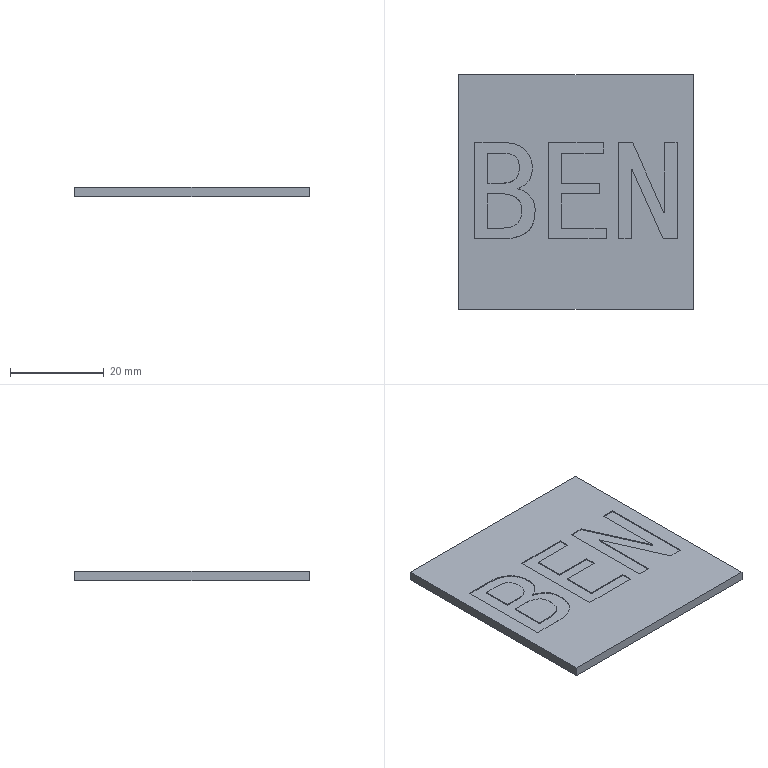Part | STEP file | lll_id1306_x_t | 1 solid | 45 faces | box 50 x 50 x 2 mm | volume 4916 mm3 | plane 38 | other 7
STEP:
#1=CARTESIAN_POINT('',(3004.59,-535.392,3.259));
#2=VERTEX_POINT('',#1);
#3=CARTESIAN_POINT('',(3007.171,-536.893,3.259));
#4=VERTEX_POINT('',#3);
#5=CARTESIAN_POINT('',(3004.59,-535.392,3.259));
#6=CARTESIAN_POINT('',(3005.552,-535.633,3.259));
#7=CARTESIAN_POINT('',(3006.406,-536.128,3.259));
#8=CARTESIAN_POINT('',(3007.171,-536.893,3.259));
#9=B_SPLINE_CURVE_WITH_KNOTS('',3,(#5,#6,#7,#8),.UNSPECIFIED.,.F.,.F.,(4,4),(0.,1.),.UNSPECIFIED.);
#10=EDGE_CURVE('',#2,#4,#9,.T.);
#11=ORIENTED_EDGE('',*,*,#10,.T.);
#12=CARTESIAN_POINT('',(2995.474,-546.065,3.259));
#13=VERTEX_POINT('',#12);
#14=CARTESIAN_POINT('',(3007.171,-536.893,3.259));
#15=CARTESIAN_POINT('',(3007.93,-537.652,3.259));
#16=CARTESIAN_POINT('',(3008.307,-538.67,3.259));
#17=CARTESIAN_POINT('',(3008.307,-542.269,3.259));
#18=CARTESIAN_POINT('',(3007.666,-543.866,3.259));
#19=CARTESIAN_POINT('',(3005.112,-545.633,3.259));
#20=CARTESIAN_POINT('',(3003.471,-546.065,3.259));
#21=CARTESIAN_POINT('',(2999.471,-546.065,3.259));
#22=CARTESIAN_POINT('',(2997.473,-546.065,3.259));
#23=CARTESIAN_POINT('',(2995.474,-546.065,3.259));
#24=B_SPLINE_CURVE_WITH_KNOTS('',3,(#14,#15,#16,#17,#18,#19,#20,#21,#22,#23),.UNSPECIFIED.,.F.,.F.,(4,2,2,2,4),(0.,0.1548,0.4366,0.7185,1.),.UNSPECIFIED.);
#25=EDGE_CURVE('',#4,#13,#24,.T.);
#26=ORIENTED_EDGE('',*,*,#25,.T.);
#27=CARTESIAN_POINT('',(2995.474,-525.556,3.259));
#28=VERTEX_POINT('',#27);
#29=CARTESIAN_POINT('',(2995.474,-535.811,3.259));
#30=DIRECTION('',(0.,1.,0.));
#31=VECTOR('',#30,1.);
#32=LINE('',#29,#31);
#33=EDGE_CURVE('',#13,#28,#32,.T.);
#34=ORIENTED_EDGE('',*,*,#33,.T.);
#35=CARTESIAN_POINT('',(2995.474,-525.556,3.259));
#36=CARTESIAN_POINT('',(2997.553,-525.556,3.259));
#37=CARTESIAN_POINT('',(2999.632,-525.556,3.259));
#38=CARTESIAN_POINT('',(3003.707,-525.556,3.259));
#39=CARTESIAN_POINT('',(3005.209,-526.074,3.259));
#40=CARTESIAN_POINT('',(3007.211,-528.154,3.259));
#41=CARTESIAN_POINT('',(3007.711,-529.391,3.259));
#42=CARTESIAN_POINT('',(3007.711,-532.271,3.259));
#43=CARTESIAN_POINT('',(3007.368,-533.333,3.259));
#44=CARTESIAN_POINT('',(3006.01,-534.691,3.259));
#45=CARTESIAN_POINT('',(3005.31,-535.15,3.259));
#46=CARTESIAN_POINT('',(3004.59,-535.392,3.259));
#47=B_SPLINE_CURVE_WITH_KNOTS('',3,(#35,#36,#37,#38,#39,#40,#41,#42,#43,#44,#45,#46),.UNSPECIFIED.,.F.,.F.,(4,2,2,2,2,4),(0.,0.2067,0.4052,0.6038,0.8023,1.),.UNSPECIFIED.);
#48=EDGE_CURVE('',#28,#2,#47,.T.);
#49=ORIENTED_EDGE('',*,*,#48,.T.);
#50=EDGE_LOOP('',(#11,#26,#34,#49));
#51=FACE_BOUND('',#50,.T.);
#52=CARTESIAN_POINT('',(3042.009,-561.065,3.259));
#53=VERTEX_POINT('',#52);
#54=CARTESIAN_POINT('',(2992.009,-561.065,3.259));
#55=VERTEX_POINT('',#54);
#56=CARTESIAN_POINT('',(3092.009,-561.065,3.259));
#57=DIRECTION('',(-1.,0.,0.));
#58=VECTOR('',#57,1.);
#59=LINE('',#56,#58);
#60=EDGE_CURVE('',#53,#55,#59,.T.);
#61=ORIENTED_EDGE('',*,*,#60,.F.);
#62=CARTESIAN_POINT('',(3042.009,-511.065,3.259));
#63=VERTEX_POINT('',#62);
#64=CARTESIAN_POINT('',(3042.009,-461.065,3.259));
#65=DIRECTION('',(0.,-1.,0.));
#66=VECTOR('',#65,1.);
#67=LINE('',#64,#66);
#68=EDGE_CURVE('',#63,#53,#67,.T.);
#69=ORIENTED_EDGE('',*,*,#68,.F.);
#70=CARTESIAN_POINT('',(2992.009,-511.065,3.259));
#71=VERTEX_POINT('',#70);
#72=CARTESIAN_POINT('',(3092.009,-511.065,3.259));
#73=DIRECTION('',(-1.,0.,0.));
#74=VECTOR('',#73,1.);
#75=LINE('',#72,#74);
#76=EDGE_CURVE('',#63,#71,#75,.T.);
#77=ORIENTED_EDGE('',*,*,#76,.T.);
#78=CARTESIAN_POINT('',(2992.009,-461.065,3.259));
#79=DIRECTION('',(0.,1.,0.));
#80=VECTOR('',#79,1.);
#81=LINE('',#78,#80);
#82=EDGE_CURVE('',#55,#71,#81,.T.);
#83=ORIENTED_EDGE('',*,*,#82,.F.);
#84=EDGE_LOOP('',(#61,#69,#77,#83));
#85=FACE_BOUND('',#84,.T.);
#86=CARTESIAN_POINT('',(3013.947,-543.787,3.259));
#87=VERTEX_POINT('',#86);
#88=CARTESIAN_POINT('',(3023.429,-543.787,3.259));
#89=VERTEX_POINT('',#88);
#90=CARTESIAN_POINT('',(3018.688,-543.787,3.259));
#91=DIRECTION('',(1.,0.,0.));
#92=VECTOR('',#91,1.);
#93=LINE('',#90,#92);
#94=EDGE_CURVE('',#87,#89,#93,.T.);
#95=ORIENTED_EDGE('',*,*,#94,.T.);
#96=CARTESIAN_POINT('',(3023.429,-546.065,3.259));
#97=VERTEX_POINT('',#96);
#98=CARTESIAN_POINT('',(3023.429,-544.926,3.259));
#99=DIRECTION('',(0.,-1.,0.));
#100=VECTOR('',#99,1.);
#101=LINE('',#98,#100);
#102=EDGE_CURVE('',#89,#97,#101,.T.);
#103=ORIENTED_EDGE('',*,*,#102,.T.);
#104=CARTESIAN_POINT('',(3011.192,-546.065,3.259));
#105=VERTEX_POINT('',#104);
#106=CARTESIAN_POINT('',(3017.31,-546.065,3.259));
#107=DIRECTION('',(-1.,0.,0.));
#108=VECTOR('',#107,1.);
#109=LINE('',#106,#108);
#110=EDGE_CURVE('',#97,#105,#109,.T.);
#111=ORIENTED_EDGE('',*,*,#110,.T.);
#112=CARTESIAN_POINT('',(3011.192,-525.556,3.259));
#113=VERTEX_POINT('',#112);
#114=CARTESIAN_POINT('',(3011.192,-535.811,3.259));
#115=DIRECTION('',(0.,1.,0.));
#116=VECTOR('',#115,1.);
#117=LINE('',#114,#116);
#118=EDGE_CURVE('',#105,#113,#117,.T.);
#119=ORIENTED_EDGE('',*,*,#118,.T.);
#120=CARTESIAN_POINT('',(3022.827,-525.556,3.259));
#121=VERTEX_POINT('',#120);
#122=CARTESIAN_POINT('',(3017.009,-525.556,3.259));
#123=DIRECTION('',(1.,0.,0.));
#124=VECTOR('',#123,1.);
#125=LINE('',#122,#124);
#126=EDGE_CURVE('',#113,#121,#125,.T.);
#127=ORIENTED_EDGE('',*,*,#126,.T.);
#128=CARTESIAN_POINT('',(3022.827,-527.834,3.259));
#129=VERTEX_POINT('',#128);
#130=CARTESIAN_POINT('',(3022.827,-526.695,3.259));
#131=DIRECTION('',(0.,-1.,0.));
#132=VECTOR('',#131,1.);
#133=LINE('',#130,#132);
#134=EDGE_CURVE('',#121,#129,#133,.T.);
#135=ORIENTED_EDGE('',*,*,#134,.T.);
#136=CARTESIAN_POINT('',(3013.947,-527.834,3.259));
#137=VERTEX_POINT('',#136);
#138=CARTESIAN_POINT('',(3018.387,-527.834,3.259));
#139=DIRECTION('',(-1.,0.,0.));
#140=VECTOR('',#139,1.);
#141=LINE('',#138,#140);
#142=EDGE_CURVE('',#129,#137,#141,.T.);
#143=ORIENTED_EDGE('',*,*,#142,.T.);
#144=CARTESIAN_POINT('',(3013.947,-534.194,3.259));
#145=VERTEX_POINT('',#144);
#146=CARTESIAN_POINT('',(3013.947,-531.014,3.259));
#147=DIRECTION('',(0.,-1.,0.));
#148=VECTOR('',#147,1.);
#149=LINE('',#146,#148);
#150=EDGE_CURVE('',#137,#145,#149,.T.);
#151=ORIENTED_EDGE('',*,*,#150,.T.);
#152=CARTESIAN_POINT('',(3022.107,-534.194,3.259));
#153=VERTEX_POINT('',#152);
#154=CARTESIAN_POINT('',(3018.027,-534.194,3.259));
#155=DIRECTION('',(1.,0.,0.));
#156=VECTOR('',#155,1.);
#157=LINE('',#154,#156);
#158=EDGE_CURVE('',#145,#153,#157,.T.);
#159=ORIENTED_EDGE('',*,*,#158,.T.);
#160=CARTESIAN_POINT('',(3022.107,-536.471,3.259));
#161=VERTEX_POINT('',#160);
#162=CARTESIAN_POINT('',(3022.107,-535.333,3.259));
#163=DIRECTION('',(0.,-1.,0.));
#164=VECTOR('',#163,1.);
#165=LINE('',#162,#164);
#166=EDGE_CURVE('',#153,#161,#165,.T.);
#167=ORIENTED_EDGE('',*,*,#166,.T.);
#168=CARTESIAN_POINT('',(3013.947,-536.471,3.259));
#169=VERTEX_POINT('',#168);
#170=CARTESIAN_POINT('',(3018.027,-536.471,3.259));
#171=DIRECTION('',(-1.,0.,0.));
#172=VECTOR('',#171,1.);
#173=LINE('',#170,#172);
#174=EDGE_CURVE('',#161,#169,#173,.T.);
#175=ORIENTED_EDGE('',*,*,#174,.T.);
#176=CARTESIAN_POINT('',(3013.947,-540.129,3.259));
#177=DIRECTION('',(0.,-1.,0.));
#178=VECTOR('',#177,1.);
#179=LINE('',#176,#178);
#180=EDGE_CURVE('',#169,#87,#179,.T.);
#181=ORIENTED_EDGE('',*,*,#180,.T.);
#182=EDGE_LOOP('',(#95,#103,#111,#119,#127,#135,#143,#151,#159,#167,#175,#181));
#183=FACE_BOUND('',#182,.T.);
#184=CARTESIAN_POINT('',(3035.783,-525.556,3.259));
#185=VERTEX_POINT('',#184);
#186=CARTESIAN_POINT('',(3038.545,-525.556,3.259));
#187=VERTEX_POINT('',#186);
#188=CARTESIAN_POINT('',(3037.164,-525.556,3.259));
#189=DIRECTION('',(1.,0.,0.));
#190=VECTOR('',#189,1.);
#191=LINE('',#188,#190);
#192=EDGE_CURVE('',#185,#187,#191,.T.);
#193=ORIENTED_EDGE('',*,*,#192,.T.);
#194=CARTESIAN_POINT('',(3038.545,-546.065,3.259));
#195=VERTEX_POINT('',#194);
#196=CARTESIAN_POINT('',(3038.545,-535.811,3.259));
#197=DIRECTION('',(0.,-1.,0.));
#198=VECTOR('',#197,1.);
#199=LINE('',#196,#198);
#200=EDGE_CURVE('',#187,#195,#199,.T.);
#201=ORIENTED_EDGE('',*,*,#200,.T.);
#202=CARTESIAN_POINT('',(3035.547,-546.065,3.259));
#203=VERTEX_POINT('',#202);
#204=CARTESIAN_POINT('',(3037.046,-546.065,3.259));
#205=DIRECTION('',(-1.,0.,0.));
#206=VECTOR('',#205,1.);
#207=LINE('',#204,#206);
#208=EDGE_CURVE('',#195,#203,#207,.T.);
#209=ORIENTED_EDGE('',*,*,#208,.T.);
#210=CARTESIAN_POINT('',(3028.945,-531.191,3.259));
#211=VERTEX_POINT('',#210);
#212=CARTESIAN_POINT('',(3032.246,-538.628,3.259));
#213=DIRECTION('',(-0.4057,0.914,0.));
#214=VECTOR('',#213,1.);
#215=LINE('',#212,#214);
#216=EDGE_CURVE('',#203,#211,#215,.T.);
#217=ORIENTED_EDGE('',*,*,#216,.T.);
#218=CARTESIAN_POINT('',(3028.827,-531.191,3.259));
#219=VERTEX_POINT('',#218);
#220=CARTESIAN_POINT('',(3028.886,-531.191,3.259));
#221=DIRECTION('',(-1.,0.,0.));
#222=VECTOR('',#221,1.);
#223=LINE('',#220,#222);
#224=EDGE_CURVE('',#211,#219,#223,.T.);
#225=ORIENTED_EDGE('',*,*,#224,.T.);
#226=CARTESIAN_POINT('',(3028.827,-546.065,3.259));
#227=VERTEX_POINT('',#226);
#228=CARTESIAN_POINT('',(3028.827,-538.628,3.259));
#229=DIRECTION('',(0.,-1.,0.));
#230=VECTOR('',#229,1.);
#231=LINE('',#228,#230);
#232=EDGE_CURVE('',#219,#227,#231,.T.);
#233=ORIENTED_EDGE('',*,*,#232,.T.);
#234=CARTESIAN_POINT('',(3026.066,-546.065,3.259));
#235=VERTEX_POINT('',#234);
#236=CARTESIAN_POINT('',(3027.447,-546.065,3.259));
#237=DIRECTION('',(-1.,0.,0.));
#238=VECTOR('',#237,1.);
#239=LINE('',#236,#238);
#240=EDGE_CURVE('',#227,#235,#239,.T.);
#241=ORIENTED_EDGE('',*,*,#240,.T.);
#242=CARTESIAN_POINT('',(3026.066,-525.556,3.259));
#243=VERTEX_POINT('',#242);
#244=CARTESIAN_POINT('',(3026.066,-535.811,3.259));
#245=DIRECTION('',(0.,1.,0.));
#246=VECTOR('',#245,1.);
#247=LINE('',#244,#246);
#248=EDGE_CURVE('',#235,#243,#247,.T.);
#249=ORIENTED_EDGE('',*,*,#248,.T.);
#250=CARTESIAN_POINT('',(3029.069,-525.556,3.259));
#251=VERTEX_POINT('',#250);
#252=CARTESIAN_POINT('',(3027.568,-525.556,3.259));
#253=DIRECTION('',(1.,0.,0.));
#254=VECTOR('',#253,1.);
#255=LINE('',#252,#254);
#256=EDGE_CURVE('',#243,#251,#255,.T.);
#257=ORIENTED_EDGE('',*,*,#256,.T.);
#258=CARTESIAN_POINT('',(3035.665,-540.43,3.259));
#259=VERTEX_POINT('',#258);
#260=CARTESIAN_POINT('',(3032.367,-532.993,3.259));
#261=DIRECTION('',(0.4054,-0.9141,0.));
#262=VECTOR('',#261,1.);
#263=LINE('',#260,#262);
#264=EDGE_CURVE('',#251,#259,#263,.T.);
#265=ORIENTED_EDGE('',*,*,#264,.T.);
#266=CARTESIAN_POINT('',(3035.783,-540.43,3.259));
#267=VERTEX_POINT('',#266);
#268=CARTESIAN_POINT('',(3035.724,-540.43,3.259));
#269=DIRECTION('',(1.,0.,0.));
#270=VECTOR('',#269,1.);
#271=LINE('',#268,#270);
#272=EDGE_CURVE('',#259,#267,#271,.T.);
#273=ORIENTED_EDGE('',*,*,#272,.T.);
#274=CARTESIAN_POINT('',(3035.783,-532.993,3.259));
#275=DIRECTION('',(0.,1.,0.));
#276=VECTOR('',#275,1.);
#277=LINE('',#274,#276);
#278=EDGE_CURVE('',#267,#185,#277,.T.);
#279=ORIENTED_EDGE('',*,*,#278,.T.);
#280=EDGE_LOOP('',(#193,#201,#209,#217,#225,#233,#241,#249,#257,#265,#273,#279));
#281=FACE_BOUND('',#280,.T.);
#282=CARTESIAN_POINT('',(3092.009,-461.065,3.259));
#283=DIRECTION('',(0.,0.,1.));
#284=DIRECTION('',(1.,0.,0.));
#285=AXIS2_PLACEMENT_3D('',#282,#283,#284);
#286=PLANE('',#285);
#287=ADVANCED_FACE('',(#51,#85,#183,#281),#286,.T.);
#288=CARTESIAN_POINT('',(3042.009,-561.065,1.259));
#289=VERTEX_POINT('',#288);
#290=CARTESIAN_POINT('',(3042.009,-561.065,179.534));
#291=DIRECTION('',(0.,0.,1.));
#292=VECTOR('',#291,1.);
#293=LINE('',#290,#292);
#294=EDGE_CURVE('',#289,#53,#293,.T.);
#295=ORIENTED_EDGE('',*,*,#294,.F.);
#296=CARTESIAN_POINT('',(3042.009,-511.065,1.259));
#297=VERTEX_POINT('',#296);
#298=CARTESIAN_POINT('',(3042.009,-461.065,1.259));
#299=DIRECTION('',(0.,-1.,0.));
#300=VECTOR('',#299,1.);
#301=LINE('',#298,#300);
#302=EDGE_CURVE('',#297,#289,#301,.T.);
#303=ORIENTED_EDGE('',*,*,#302,.F.);
#304=CARTESIAN_POINT('',(3042.009,-511.065,2.109));
#305=DIRECTION('',(0.,0.,-1.));
#306=VECTOR('',#305,1.);
#307=LINE('',#304,#306);
#308=EDGE_CURVE('',#63,#297,#307,.T.);
#309=ORIENTED_EDGE('',*,*,#308,.F.);
#310=ORIENTED_EDGE('',*,*,#68,.T.);
#311=EDGE_LOOP('',(#295,#303,#309,#310));
#312=FACE_OUTER_BOUND('',#311,.T.);
#313=CARTESIAN_POINT('',(3042.009,-536.065,2.259));
#314=DIRECTION('',(1.,0.,0.));
#315=DIRECTION('',(0.,0.,-1.));
#316=AXIS2_PLACEMENT_3D('',#313,#314,#315);
#317=PLANE('',#316);
#318=ADVANCED_FACE('',(#312),#317,.T.);
#319=CARTESIAN_POINT('',(2992.009,-511.065,1.259));
#320=VERTEX_POINT('',#319);
#321=CARTESIAN_POINT('',(2992.009,-511.065,2.109));
#322=DIRECTION('',(0.,0.,1.));
#323=VECTOR('',#322,1.);
#324=LINE('',#321,#323);
#325=EDGE_CURVE('',#320,#71,#324,.T.);
#326=ORIENTED_EDGE('',*,*,#325,.F.);
#327=CARTESIAN_POINT('',(2992.009,-561.065,1.259));
#328=VERTEX_POINT('',#327);
#329=CARTESIAN_POINT('',(2992.009,-461.065,1.259));
#330=DIRECTION('',(0.,-1.,0.));
#331=VECTOR('',#330,1.);
#332=LINE('',#329,#331);
#333=EDGE_CURVE('',#320,#328,#332,.T.);
#334=ORIENTED_EDGE('',*,*,#333,.T.);
#335=CARTESIAN_POINT('',(2992.009,-561.065,179.534));
#336=DIRECTION('',(0.,0.,1.));
#337=VECTOR('',#336,1.);
#338=LINE('',#335,#337);
#339=EDGE_CURVE('',#328,#55,#338,.T.);
#340=ORIENTED_EDGE('',*,*,#339,.T.);
#341=ORIENTED_EDGE('',*,*,#82,.T.);
#342=EDGE_LOOP('',(#326,#334,#340,#341));
#343=FACE_OUTER_BOUND('',#342,.T.);
#344=CARTESIAN_POINT('',(2992.009,-511.065,2.109));
#345=DIRECTION('',(1.,0.,0.));
#346=DIRECTION('',(0.,0.,-1.));
#347=AXIS2_PLACEMENT_3D('',#344,#345,#346);
#348=PLANE('',#347);
#349=ADVANCED_FACE('',(#343),#348,.F.);
#350=ORIENTED_EDGE('',*,*,#76,.F.);
#351=ORIENTED_EDGE('',*,*,#308,.T.);
#352=CARTESIAN_POINT('',(1532.009,-511.065,1.259));
#353=DIRECTION('',(1.,0.,0.));
#354=VECTOR('',#353,1.);
#355=LINE('',#352,#354);
#356=EDGE_CURVE('',#320,#297,#355,.T.);
#357=ORIENTED_EDGE('',*,*,#356,.F.);
#358=ORIENTED_EDGE('',*,*,#325,.T.);
#359=EDGE_LOOP('',(#350,#351,#357,#358));
#360=FACE_OUTER_BOUND('',#359,.T.);
#361=CARTESIAN_POINT('',(3042.009,-511.065,2.109));
#362=DIRECTION('',(0.,1.,0.));
#363=DIRECTION('',(0.,0.,1.));
#364=AXIS2_PLACEMENT_3D('',#361,#362,#363);
#365=PLANE('',#364);
#366=ADVANCED_FACE('',(#360),#365,.T.);
#367=CARTESIAN_POINT('',(-4224.12,-561.065,1.259));
#368=DIRECTION('',(1.,0.,0.));
#369=VECTOR('',#368,1.);
#370=LINE('',#367,#369);
#371=EDGE_CURVE('',#328,#289,#370,.T.);
#372=ORIENTED_EDGE('',*,*,#371,.T.);
#373=ORIENTED_EDGE('',*,*,#294,.T.);
#374=ORIENTED_EDGE('',*,*,#60,.T.);
#375=ORIENTED_EDGE('',*,*,#339,.F.);
#376=EDGE_LOOP('',(#372,#373,#374,#375));
#377=FACE_OUTER_BOUND('',#376,.T.);
#378=CARTESIAN_POINT('',(-4224.12,-561.065,179.534));
#379=DIRECTION('',(0.,-1.,0.));
#380=DIRECTION('',(0.,0.,-1.));
#381=AXIS2_PLACEMENT_3D('',#378,#379,#380);
#382=PLANE('',#381);
#383=ADVANCED_FACE('',(#377),#382,.T.);
#384=ORIENTED_EDGE('',*,*,#356,.T.);
#385=ORIENTED_EDGE('',*,*,#302,.T.);
#386=ORIENTED_EDGE('',*,*,#371,.F.);
#387=ORIENTED_EDGE('',*,*,#333,.F.);
#388=EDGE_LOOP('',(#384,#385,#386,#387));
#389=FACE_OUTER_BOUND('',#388,.T.);
#390=CARTESIAN_POINT('',(1532.009,-461.065,1.259));
#391=DIRECTION('',(0.,0.,-1.));
#392=DIRECTION('',(-1.,0.,0.));
#393=AXIS2_PLACEMENT_3D('',#390,#391,#392);
#394=PLANE('',#393);
#395=ADVANCED_FACE('',(#389),#394,.T.);
#396=ORIENTED_EDGE('',*,*,#102,.F.);
#397=CARTESIAN_POINT('',(3023.429,-543.787,3.059));
#398=VERTEX_POINT('',#397);
#399=CARTESIAN_POINT('',(3023.429,-543.787,3.059));
#400=DIRECTION('',(0.,0.,-1.));
#401=VECTOR('',#400,1.);
#402=LINE('',#399,#401);
#403=EDGE_CURVE('',#89,#398,#402,.T.);
#404=ORIENTED_EDGE('',*,*,#403,.T.);
#405=CARTESIAN_POINT('',(3023.429,-546.065,3.059));
#406=VERTEX_POINT('',#405);
#407=CARTESIAN_POINT('',(3023.429,-544.926,3.059));
#408=DIRECTION('',(0.,1.,0.));
#409=VECTOR('',#408,1.);
#410=LINE('',#407,#409);
#411=EDGE_CURVE('',#406,#398,#410,.T.);
#412=ORIENTED_EDGE('',*,*,#411,.F.);
#413=CARTESIAN_POINT('',(3023.429,-546.065,3.059));
#414=DIRECTION('',(0.,0.,-1.));
#415=VECTOR('',#414,1.);
#416=LINE('',#413,#415);
#417=EDGE_CURVE('',#97,#406,#416,.T.);
#418=ORIENTED_EDGE('',*,*,#417,.F.);
#419=EDGE_LOOP('',(#396,#404,#412,#418));
#420=FACE_OUTER_BOUND('',#419,.T.);
#421=CARTESIAN_POINT('',(3023.429,-543.787,3.059));
#422=DIRECTION('',(-1.,0.,0.));
#423=DIRECTION('',(0.,0.,1.));
#424=AXIS2_PLACEMENT_3D('',#421,#422,#423);
#425=PLANE('',#424);
#426=ADVANCED_FACE('',(#420),#425,.T.);
#427=ORIENTED_EDGE('',*,*,#110,.F.);
#428=ORIENTED_EDGE('',*,*,#417,.T.);
#429=CARTESIAN_POINT('',(3011.192,-546.065,3.059));
#430=VERTEX_POINT('',#429);
#431=CARTESIAN_POINT('',(3017.31,-546.065,3.059));
#432=DIRECTION('',(1.,0.,0.));
#433=VECTOR('',#432,1.);
#434=LINE('',#431,#433);
#435=EDGE_CURVE('',#430,#406,#434,.T.);
#436=ORIENTED_EDGE('',*,*,#435,.F.);
#437=CARTESIAN_POINT('',(3011.192,-546.065,3.059));
#438=DIRECTION('',(0.,0.,-1.));
#439=VECTOR('',#438,1.);
#440=LINE('',#437,#439);
#441=EDGE_CURVE('',#105,#430,#440,.T.);
#442=ORIENTED_EDGE('',*,*,#441,.F.);
#443=EDGE_LOOP('',(#427,#428,#436,#442));
#444=FACE_OUTER_BOUND('',#443,.T.);
#445=CARTESIAN_POINT('',(3023.429,-546.065,3.059));
#446=DIRECTION('',(0.,1.,0.));
#447=DIRECTION('',(0.,0.,1.));
#448=AXIS2_PLACEMENT_3D('',#445,#446,#447);
#449=PLANE('',#448);
#450=ADVANCED_FACE('',(#444),#449,.T.);
#451=ORIENTED_EDGE('',*,*,#118,.F.);
#452=ORIENTED_EDGE('',*,*,#441,.T.);
#453=CARTESIAN_POINT('',(3011.192,-525.556,3.059));
#454=VERTEX_POINT('',#453);
#455=CARTESIAN_POINT('',(3011.192,-535.811,3.059));
#456=DIRECTION('',(0.,-1.,0.));
#457=VECTOR('',#456,1.);
#458=LINE('',#455,#457);
#459=EDGE_CURVE('',#454,#430,#458,.T.);
#460=ORIENTED_EDGE('',*,*,#459,.F.);
#461=CARTESIAN_POINT('',(3011.192,-525.556,3.059));
#462=DIRECTION('',(0.,0.,-1.));
#463=VECTOR('',#462,1.);
#464=LINE('',#461,#463);
#465=EDGE_CURVE('',#113,#454,#464,.T.);
#466=ORIENTED_EDGE('',*,*,#465,.F.);
#467=EDGE_LOOP('',(#451,#452,#460,#466));
#468=FACE_OUTER_BOUND('',#467,.T.);
#469=CARTESIAN_POINT('',(3011.192,-546.065,3.059));
#470=DIRECTION('',(1.,0.,0.));
#471=DIRECTION('',(0.,0.,-1.));
#472=AXIS2_PLACEMENT_3D('',#469,#470,#471);
#473=PLANE('',#472);
#474=ADVANCED_FACE('',(#468),#473,.T.);
#475=ORIENTED_EDGE('',*,*,#126,.F.);
#476=ORIENTED_EDGE('',*,*,#465,.T.);
#477=CARTESIAN_POINT('',(3022.827,-525.556,3.059));
#478=VERTEX_POINT('',#477);
#479=CARTESIAN_POINT('',(3017.009,-525.556,3.059));
#480=DIRECTION('',(-1.,0.,0.));
#481=VECTOR('',#480,1.);
#482=LINE('',#479,#481);
#483=EDGE_CURVE('',#478,#454,#482,.T.);
#484=ORIENTED_EDGE('',*,*,#483,.F.);
#485=CARTESIAN_POINT('',(3022.827,-525.556,3.059));
#486=DIRECTION('',(0.,0.,-1.));
#487=VECTOR('',#486,1.);
#488=LINE('',#485,#487);
#489=EDGE_CURVE('',#121,#478,#488,.T.);
#490=ORIENTED_EDGE('',*,*,#489,.F.);
#491=EDGE_LOOP('',(#475,#476,#484,#490));
#492=FACE_OUTER_BOUND('',#491,.T.);
#493=CARTESIAN_POINT('',(3011.192,-525.556,3.059));
#494=DIRECTION('',(0.,-1.,0.));
#495=DIRECTION('',(0.,0.,-1.));
#496=AXIS2_PLACEMENT_3D('',#493,#494,#495);
#497=PLANE('',#496);
#498=ADVANCED_FACE('',(#492),#497,.T.);
#499=ORIENTED_EDGE('',*,*,#134,.F.);
#500=ORIENTED_EDGE('',*,*,#489,.T.);
#501=CARTESIAN_POINT('',(3022.827,-527.834,3.059));
#502=VERTEX_POINT('',#501);
#503=CARTESIAN_POINT('',(3022.827,-526.695,3.059));
#504=DIRECTION('',(0.,1.,0.));
#505=VECTOR('',#504,1.);
#506=LINE('',#503,#505);
#507=EDGE_CURVE('',#502,#478,#506,.T.);
#508=ORIENTED_EDGE('',*,*,#507,.F.);
#509=CARTESIAN_POINT('',(3022.827,-527.834,3.059));
#510=DIRECTION('',(0.,0.,-1.));
#511=VECTOR('',#510,1.);
#512=LINE('',#509,#511);
#513=EDGE_CURVE('',#129,#502,#512,.T.);
#514=ORIENTED_EDGE('',*,*,#513,.F.);
#515=EDGE_LOOP('',(#499,#500,#508,#514));
#516=FACE_OUTER_BOUND('',#515,.T.);
#517=CARTESIAN_POINT('',(3022.827,-525.556,3.059));
#518=DIRECTION('',(-1.,0.,0.));
#519=DIRECTION('',(0.,0.,1.));
#520=AXIS2_PLACEMENT_3D('',#517,#518,#519);
#521=PLANE('',#520);
#522=ADVANCED_FACE('',(#516),#521,.T.);
#523=ORIENTED_EDGE('',*,*,#142,.F.);
#524=ORIENTED_EDGE('',*,*,#513,.T.);
#525=CARTESIAN_POINT('',(3013.947,-527.834,3.059));
#526=VERTEX_POINT('',#525);
#527=CARTESIAN_POINT('',(3018.387,-527.834,3.059));
#528=DIRECTION('',(1.,0.,0.));
#529=VECTOR('',#528,1.);
#530=LINE('',#527,#529);
#531=EDGE_CURVE('',#526,#502,#530,.T.);
#532=ORIENTED_EDGE('',*,*,#531,.F.);
#533=CARTESIAN_POINT('',(3013.947,-527.834,3.059));
#534=DIRECTION('',(0.,0.,-1.));
#535=VECTOR('',#534,1.);
#536=LINE('',#533,#535);
#537=EDGE_CURVE('',#137,#526,#536,.T.);
#538=ORIENTED_EDGE('',*,*,#537,.F.);
#539=EDGE_LOOP('',(#523,#524,#532,#538));
#540=FACE_OUTER_BOUND('',#539,.T.);
#541=CARTESIAN_POINT('',(3022.827,-527.834,3.059));
#542=DIRECTION('',(0.,1.,0.));
#543=DIRECTION('',(0.,0.,1.));
#544=AXIS2_PLACEMENT_3D('',#541,#542,#543);
#545=PLANE('',#544);
#546=ADVANCED_FACE('',(#540),#545,.T.);
#547=ORIENTED_EDGE('',*,*,#150,.F.);
#548=ORIENTED_EDGE('',*,*,#537,.T.);
#549=CARTESIAN_POINT('',(3013.947,-534.194,3.059));
#550=VERTEX_POINT('',#549);
#551=CARTESIAN_POINT('',(3013.947,-531.014,3.059));
#552=DIRECTION('',(0.,1.,0.));
#553=VECTOR('',#552,1.);
#554=LINE('',#551,#553);
#555=EDGE_CURVE('',#550,#526,#554,.T.);
#556=ORIENTED_EDGE('',*,*,#555,.F.);
#557=CARTESIAN_POINT('',(3013.947,-534.194,3.059));
#558=DIRECTION('',(0.,0.,-1.));
#559=VECTOR('',#558,1.);
#560=LINE('',#557,#559);
#561=EDGE_CURVE('',#145,#550,#560,.T.);
#562=ORIENTED_EDGE('',*,*,#561,.F.);
#563=EDGE_LOOP('',(#547,#548,#556,#562));
#564=FACE_OUTER_BOUND('',#563,.T.);
#565=CARTESIAN_POINT('',(3013.947,-527.834,3.059));
#566=DIRECTION('',(-1.,0.,0.));
#567=DIRECTION('',(0.,0.,1.));
#568=AXIS2_PLACEMENT_3D('',#565,#566,#567);
#569=PLANE('',#568);
#570=ADVANCED_FACE('',(#564),#569,.T.);
#571=ORIENTED_EDGE('',*,*,#158,.F.);
#572=ORIENTED_EDGE('',*,*,#561,.T.);
#573=CARTESIAN_POINT('',(3022.107,-534.194,3.059));
#574=VERTEX_POINT('',#573);
#575=CARTESIAN_POINT('',(3018.027,-534.194,3.059));
#576=DIRECTION('',(-1.,0.,0.));
#577=VECTOR('',#576,1.);
#578=LINE('',#575,#577);
#579=EDGE_CURVE('',#574,#550,#578,.T.);
#580=ORIENTED_EDGE('',*,*,#579,.F.);
#581=CARTESIAN_POINT('',(3022.107,-534.194,3.059));
#582=DIRECTION('',(0.,0.,-1.));
#583=VECTOR('',#582,1.);
#584=LINE('',#581,#583);
#585=EDGE_CURVE('',#153,#574,#584,.T.);
#586=ORIENTED_EDGE('',*,*,#585,.F.);
#587=EDGE_LOOP('',(#571,#572,#580,#586));
#588=FACE_OUTER_BOUND('',#587,.T.);
#589=CARTESIAN_POINT('',(3013.947,-534.194,3.059));
#590=DIRECTION('',(0.,-1.,0.));
#591=DIRECTION('',(0.,0.,-1.));
#592=AXIS2_PLACEMENT_3D('',#589,#590,#591);
#593=PLANE('',#592);
#594=ADVANCED_FACE('',(#588),#593,.T.);
#595=ORIENTED_EDGE('',*,*,#166,.F.);
#596=ORIENTED_EDGE('',*,*,#585,.T.);
#597=CARTESIAN_POINT('',(3022.107,-536.471,3.059));
#598=VERTEX_POINT('',#597);
#599=CARTESIAN_POINT('',(3022.107,-535.333,3.059));
#600=DIRECTION('',(0.,1.,0.));
#601=VECTOR('',#600,1.);
#602=LINE('',#599,#601);
#603=EDGE_CURVE('',#598,#574,#602,.T.);
#604=ORIENTED_EDGE('',*,*,#603,.F.);
#605=CARTESIAN_POINT('',(3022.107,-536.471,3.059));
#606=DIRECTION('',(0.,0.,-1.));
#607=VECTOR('',#606,1.);
#608=LINE('',#605,#607);
#609=EDGE_CURVE('',#161,#598,#608,.T.);
#610=ORIENTED_EDGE('',*,*,#609,.F.);
#611=EDGE_LOOP('',(#595,#596,#604,#610));
#612=FACE_OUTER_BOUND('',#611,.T.);
#613=CARTESIAN_POINT('',(3022.107,-534.194,3.059));
#614=DIRECTION('',(-1.,0.,0.));
#615=DIRECTION('',(0.,0.,1.));
#616=AXIS2_PLACEMENT_3D('',#613,#614,#615);
#617=PLANE('',#616);
#618=ADVANCED_FACE('',(#612),#617,.T.);
#619=ORIENTED_EDGE('',*,*,#174,.F.);
#620=ORIENTED_EDGE('',*,*,#609,.T.);
#621=CARTESIAN_POINT('',(3013.947,-536.471,3.059));
#622=VERTEX_POINT('',#621);
#623=CARTESIAN_POINT('',(3018.027,-536.471,3.059));
#624=DIRECTION('',(1.,0.,0.));
#625=VECTOR('',#624,1.);
#626=LINE('',#623,#625);
#627=EDGE_CURVE('',#622,#598,#626,.T.);
#628=ORIENTED_EDGE('',*,*,#627,.F.);
#629=CARTESIAN_POINT('',(3013.947,-536.471,3.059));
#630=DIRECTION('',(0.,0.,-1.));
#631=VECTOR('',#630,1.);
#632=LINE('',#629,#631);
#633=EDGE_CURVE('',#169,#622,#632,.T.);
#634=ORIENTED_EDGE('',*,*,#633,.F.);
#635=EDGE_LOOP('',(#619,#620,#628,#634));
#636=FACE_OUTER_BOUND('',#635,.T.);
#637=CARTESIAN_POINT('',(3022.107,-536.471,3.059));
#638=DIRECTION('',(0.,1.,0.));
#639=DIRECTION('',(0.,0.,1.));
#640=AXIS2_PLACEMENT_3D('',#637,#638,#639);
#641=PLANE('',#640);
#642=ADVANCED_FACE('',(#636),#641,.T.);
#643=ORIENTED_EDGE('',*,*,#180,.F.);
#644=ORIENTED_EDGE('',*,*,#633,.T.);
#645=CARTESIAN_POINT('',(3013.947,-543.787,3.059));
#646=VERTEX_POINT('',#645);
#647=CARTESIAN_POINT('',(3013.947,-540.129,3.059));
#648=DIRECTION('',(0.,1.,0.));
#649=VECTOR('',#648,1.);
#650=LINE('',#647,#649);
#651=EDGE_CURVE('',#646,#622,#650,.T.);
#652=ORIENTED_EDGE('',*,*,#651,.F.);
#653=CARTESIAN_POINT('',(3013.947,-543.787,3.059));
#654=DIRECTION('',(0.,0.,-1.));
#655=VECTOR('',#654,1.);
#656=LINE('',#653,#655);
#657=EDGE_CURVE('',#87,#646,#656,.T.);
#658=ORIENTED_EDGE('',*,*,#657,.F.);
#659=EDGE_LOOP('',(#643,#644,#652,#658));
#660=FACE_OUTER_BOUND('',#659,.T.);
#661=CARTESIAN_POINT('',(3013.947,-536.471,3.059));
#662=DIRECTION('',(-1.,0.,0.));
#663=DIRECTION('',(0.,0.,1.));
#664=AXIS2_PLACEMENT_3D('',#661,#662,#663);
#665=PLANE('',#664);
#666=ADVANCED_FACE('',(#660),#665,.T.);
#667=ORIENTED_EDGE('',*,*,#94,.F.);
#668=ORIENTED_EDGE('',*,*,#657,.T.);
#669=CARTESIAN_POINT('',(3018.688,-543.787,3.059));
#670=DIRECTION('',(-1.,0.,0.));
#671=VECTOR('',#670,1.);
#672=LINE('',#669,#671);
#673=EDGE_CURVE('',#398,#646,#672,.T.);
#674=ORIENTED_EDGE('',*,*,#673,.F.);
#675=ORIENTED_EDGE('',*,*,#403,.F.);
#676=EDGE_LOOP('',(#667,#668,#674,#675));
#677=FACE_OUTER_BOUND('',#676,.T.);
#678=CARTESIAN_POINT('',(3013.947,-543.787,3.059));
#679=DIRECTION('',(0.,-1.,0.));
#680=DIRECTION('',(0.,0.,-1.));
#681=AXIS2_PLACEMENT_3D('',#678,#679,#680);
#682=PLANE('',#681);
#683=ADVANCED_FACE('',(#677),#682,.T.);
#684=ORIENTED_EDGE('',*,*,#411,.T.);
#685=ORIENTED_EDGE('',*,*,#673,.T.);
#686=ORIENTED_EDGE('',*,*,#651,.T.);
#687=ORIENTED_EDGE('',*,*,#627,.T.);
#688=ORIENTED_EDGE('',*,*,#603,.T.);
#689=ORIENTED_EDGE('',*,*,#579,.T.);
#690=ORIENTED_EDGE('',*,*,#555,.T.);
#691=ORIENTED_EDGE('',*,*,#531,.T.);
#692=ORIENTED_EDGE('',*,*,#507,.T.);
#693=ORIENTED_EDGE('',*,*,#483,.T.);
#694=ORIENTED_EDGE('',*,*,#459,.T.);
#695=ORIENTED_EDGE('',*,*,#435,.T.);
#696=EDGE_LOOP('',(#684,#685,#686,#687,#688,#689,#690,#691,#692,#693,#694,#695));
#697=FACE_OUTER_BOUND('',#696,.T.);
#698=CARTESIAN_POINT('',(3023.429,-544.926,3.059));
#699=DIRECTION('',(0.,0.,1.));
#700=DIRECTION('',(1.,0.,0.));
#701=AXIS2_PLACEMENT_3D('',#698,#699,#700);
#702=PLANE('',#701);
#703=ADVANCED_FACE('',(#697),#702,.T.);
#704=CARTESIAN_POINT('',(3004.292,-542.95,3.259));
#705=VERTEX_POINT('',#704);
#706=CARTESIAN_POINT('',(2998.23,-536.471,3.259));
#707=VERTEX_POINT('',#706);
#708=CARTESIAN_POINT('',(3004.292,-542.95,3.259));
#709=CARTESIAN_POINT('',(3005.051,-542.387,3.259));
#710=CARTESIAN_POINT('',(3005.428,-541.386,3.259));
#711=CARTESIAN_POINT('',(3005.428,-538.67,3.259));
#712=CARTESIAN_POINT('',(3005.012,-537.77,3.259));
#713=CARTESIAN_POINT('',(3003.326,-536.737,3.259));
#714=CARTESIAN_POINT('',(3002.391,-536.471,3.259));
#715=CARTESIAN_POINT('',(3000.311,-536.471,3.259));
#716=CARTESIAN_POINT('',(2999.27,-536.471,3.259));
#717=CARTESIAN_POINT('',(2998.23,-536.471,3.259));
#718=B_SPLINE_CURVE_WITH_KNOTS('',3,(#708,#709,#710,#711,#712,#713,#714,#715,#716,#717),.UNSPECIFIED.,.F.,.F.,(4,2,2,2,4),(0.,0.2735,0.5159,0.758,1.),.UNSPECIFIED.);
#719=EDGE_CURVE('',#705,#707,#718,.T.);
#720=ORIENTED_EDGE('',*,*,#719,.F.);
#721=CARTESIAN_POINT('',(3004.292,-542.95,3.059));
#722=VERTEX_POINT('',#721);
#723=CARTESIAN_POINT('',(3004.292,-542.95,3.059));
#724=DIRECTION('',(0.,0.,-1.));
#725=VECTOR('',#724,1.);
#726=LINE('',#723,#725);
#727=EDGE_CURVE('',#705,#722,#726,.T.);
#728=ORIENTED_EDGE('',*,*,#727,.T.);
#729=CARTESIAN_POINT('',(2998.23,-536.471,3.059));
#730=VERTEX_POINT('',#729);
#731=CARTESIAN_POINT('',(2998.23,-536.471,3.059));
#732=CARTESIAN_POINT('',(2999.27,-536.471,3.059));
#733=CARTESIAN_POINT('',(3000.311,-536.471,3.059));
#734=CARTESIAN_POINT('',(3002.391,-536.471,3.059));
#735=CARTESIAN_POINT('',(3003.326,-536.737,3.059));
#736=CARTESIAN_POINT('',(3005.012,-537.77,3.059));
#737=CARTESIAN_POINT('',(3005.428,-538.67,3.059));
#738=CARTESIAN_POINT('',(3005.428,-541.386,3.059));
#739=CARTESIAN_POINT('',(3005.051,-542.387,3.059));
#740=CARTESIAN_POINT('',(3004.292,-542.95,3.059));
#741=B_SPLINE_CURVE_WITH_KNOTS('',3,(#731,#732,#733,#734,#735,#736,#737,#738,#739,#740),.UNSPECIFIED.,.F.,.F.,(4,2,2,2,4),(0.,0.242,0.4841,0.7265,1.),.UNSPECIFIED.);
#742=EDGE_CURVE('',#730,#722,#741,.T.);
#743=ORIENTED_EDGE('',*,*,#742,.F.);
#744=CARTESIAN_POINT('',(2998.23,-536.471,3.059));
#745=DIRECTION('',(0.,0.,-1.));
#746=VECTOR('',#745,1.);
#747=LINE('',#744,#746);
#748=EDGE_CURVE('',#707,#730,#747,.T.);
#749=ORIENTED_EDGE('',*,*,#748,.F.);
#750=EDGE_LOOP('',(#720,#728,#743,#749));
#751=FACE_OUTER_BOUND('',#750,.T.);
#752=CARTESIAN_POINT('',(3004.292,-542.95,3.059));
#753=CARTESIAN_POINT('',(3005.051,-542.387,3.059));
#754=CARTESIAN_POINT('',(3005.428,-541.386,3.059));
#755=CARTESIAN_POINT('',(3005.428,-538.67,3.059));
#756=CARTESIAN_POINT('',(3005.012,-537.77,3.059));
#757=CARTESIAN_POINT('',(3003.326,-536.737,3.059));
#758=CARTESIAN_POINT('',(3002.391,-536.471,3.059));
#759=CARTESIAN_POINT('',(3000.311,-536.471,3.059));
#760=CARTESIAN_POINT('',(2999.27,-536.471,3.059));
#761=CARTESIAN_POINT('',(2998.23,-536.471,3.059));
#762=B_SPLINE_CURVE_WITH_KNOTS('',3,(#752,#753,#754,#755,#756,#757,#758,#759,#760,#761),.UNSPECIFIED.,.F.,.F.,(4,2,2,2,4),(0.,0.2735,0.5159,0.758,1.),.UNSPECIFIED.);
#763=DIRECTION('',(0.,0.,1.));
#764=VECTOR('',#763,1.);
#765=SURFACE_OF_LINEAR_EXTRUSION('',#762,#764);
#766=ADVANCED_FACE('',(#751),#765,.T.);
#767=CARTESIAN_POINT('',(2998.23,-543.787,3.259));
#768=VERTEX_POINT('',#767);
#769=CARTESIAN_POINT('',(2998.23,-540.129,3.259));
#770=DIRECTION('',(0.,-1.,0.));
#771=VECTOR('',#770,1.);
#772=LINE('',#769,#771);
#773=EDGE_CURVE('',#707,#768,#772,.T.);
#774=ORIENTED_EDGE('',*,*,#773,.F.);
#775=ORIENTED_EDGE('',*,*,#748,.T.);
#776=CARTESIAN_POINT('',(2998.23,-543.787,3.059));
#777=VERTEX_POINT('',#776);
#778=CARTESIAN_POINT('',(2998.23,-540.129,3.059));
#779=DIRECTION('',(0.,1.,0.));
#780=VECTOR('',#779,1.);
#781=LINE('',#778,#780);
#782=EDGE_CURVE('',#777,#730,#781,.T.);
#783=ORIENTED_EDGE('',*,*,#782,.F.);
#784=CARTESIAN_POINT('',(2998.23,-543.787,3.059));
#785=DIRECTION('',(0.,0.,-1.));
#786=VECTOR('',#785,1.);
#787=LINE('',#784,#786);
#788=EDGE_CURVE('',#768,#777,#787,.T.);
#789=ORIENTED_EDGE('',*,*,#788,.F.);
#790=EDGE_LOOP('',(#774,#775,#783,#789));
#791=FACE_OUTER_BOUND('',#790,.T.);
#792=CARTESIAN_POINT('',(2998.23,-536.471,3.059));
#793=DIRECTION('',(-1.,0.,0.));
#794=DIRECTION('',(0.,0.,1.));
#795=AXIS2_PLACEMENT_3D('',#792,#793,#794);
#796=PLANE('',#795);
#797=ADVANCED_FACE('',(#791),#796,.T.);
#798=CARTESIAN_POINT('',(3003.988,-533.412,3.259));
#799=VERTEX_POINT('',#798);
#800=CARTESIAN_POINT('',(2998.23,-527.834,3.259));
#801=VERTEX_POINT('',#800);
#802=CARTESIAN_POINT('',(3003.988,-533.412,3.259));
#803=CARTESIAN_POINT('',(3004.629,-532.895,3.259));
#804=CARTESIAN_POINT('',(3004.95,-532.034,3.259));
#805=CARTESIAN_POINT('',(3004.95,-529.791,3.259));
#806=CARTESIAN_POINT('',(3004.652,-529.031,3.259));
#807=CARTESIAN_POINT('',(3003.448,-528.075,3.259));
#808=CARTESIAN_POINT('',(3002.712,-527.834,3.259));
#809=CARTESIAN_POINT('',(3000.629,-527.834,3.259));
#810=CARTESIAN_POINT('',(2999.43,-527.834,3.259));
#811=CARTESIAN_POINT('',(2998.23,-527.834,3.259));
#812=B_SPLINE_CURVE_WITH_KNOTS('',3,(#802,#803,#804,#805,#806,#807,#808,#809,#810,#811),.UNSPECIFIED.,.F.,.F.,(4,2,2,2,4),(0.,0.2562,0.4776,0.6991,1.),.UNSPECIFIED.);
#813=EDGE_CURVE('',#799,#801,#812,.T.);
#814=ORIENTED_EDGE('',*,*,#813,.F.);
#815=CARTESIAN_POINT('',(3003.988,-533.412,3.059));
#816=VERTEX_POINT('',#815);
#817=CARTESIAN_POINT('',(3003.988,-533.412,3.059));
#818=DIRECTION('',(0.,0.,-1.));
#819=VECTOR('',#818,1.);
#820=LINE('',#817,#819);
#821=EDGE_CURVE('',#799,#816,#820,.T.);
#822=ORIENTED_EDGE('',*,*,#821,.T.);
#823=CARTESIAN_POINT('',(2998.23,-527.834,3.059));
#824=VERTEX_POINT('',#823);
#825=CARTESIAN_POINT('',(2998.23,-527.834,3.059));
#826=CARTESIAN_POINT('',(2999.43,-527.834,3.059));
#827=CARTESIAN_POINT('',(3000.629,-527.834,3.059));
#828=CARTESIAN_POINT('',(3002.712,-527.834,3.059));
#829=CARTESIAN_POINT('',(3003.448,-528.075,3.059));
#830=CARTESIAN_POINT('',(3004.652,-529.031,3.059));
#831=CARTESIAN_POINT('',(3004.95,-529.791,3.059));
#832=CARTESIAN_POINT('',(3004.95,-532.034,3.059));
#833=CARTESIAN_POINT('',(3004.629,-532.895,3.059));
#834=CARTESIAN_POINT('',(3003.988,-533.412,3.059));
#835=B_SPLINE_CURVE_WITH_KNOTS('',3,(#825,#826,#827,#828,#829,#830,#831,#832,#833,#834),.UNSPECIFIED.,.F.,.F.,(4,2,2,2,4),(0.,0.3009,0.5224,0.7438,1.),.UNSPECIFIED.);
#836=EDGE_CURVE('',#824,#816,#835,.T.);
#837=ORIENTED_EDGE('',*,*,#836,.F.);
#838=CARTESIAN_POINT('',(2998.23,-527.834,3.059));
#839=DIRECTION('',(0.,0.,-1.));
#840=VECTOR('',#839,1.);
#841=LINE('',#838,#840);
#842=EDGE_CURVE('',#801,#824,#841,.T.);
#843=ORIENTED_EDGE('',*,*,#842,.F.);
#844=EDGE_LOOP('',(#814,#822,#837,#843));
#845=FACE_OUTER_BOUND('',#844,.T.);
#846=CARTESIAN_POINT('',(3003.988,-533.412,3.059));
#847=CARTESIAN_POINT('',(3004.629,-532.895,3.059));
#848=CARTESIAN_POINT('',(3004.95,-532.034,3.059));
#849=CARTESIAN_POINT('',(3004.95,-529.791,3.059));
#850=CARTESIAN_POINT('',(3004.652,-529.031,3.059));
#851=CARTESIAN_POINT('',(3003.448,-528.075,3.059));
#852=CARTESIAN_POINT('',(3002.712,-527.834,3.059));
#853=CARTESIAN_POINT('',(3000.629,-527.834,3.059));
#854=CARTESIAN_POINT('',(2999.43,-527.834,3.059));
#855=CARTESIAN_POINT('',(2998.23,-527.834,3.059));
#856=B_SPLINE_CURVE_WITH_KNOTS('',3,(#846,#847,#848,#849,#850,#851,#852,#853,#854,#855),.UNSPECIFIED.,.F.,.F.,(4,2,2,2,4),(0.,0.2562,0.4776,0.6991,1.),.UNSPECIFIED.);
#857=DIRECTION('',(0.,0.,1.));
#858=VECTOR('',#857,1.);
#859=SURFACE_OF_LINEAR_EXTRUSION('',#856,#858);
#860=ADVANCED_FACE('',(#845),#859,.T.);
#861=CARTESIAN_POINT('',(2998.23,-534.194,3.259));
#862=VERTEX_POINT('',#861);
#863=CARTESIAN_POINT('',(2998.23,-531.014,3.259));
#864=DIRECTION('',(0.,-1.,0.));
#865=VECTOR('',#864,1.);
#866=LINE('',#863,#865);
#867=EDGE_CURVE('',#801,#862,#866,.T.);
#868=ORIENTED_EDGE('',*,*,#867,.F.);
#869=ORIENTED_EDGE('',*,*,#842,.T.);
#870=CARTESIAN_POINT('',(2998.23,-534.194,3.059));
#871=VERTEX_POINT('',#870);
#872=CARTESIAN_POINT('',(2998.23,-531.014,3.059));
#873=DIRECTION('',(0.,1.,0.));
#874=VECTOR('',#873,1.);
#875=LINE('',#872,#874);
#876=EDGE_CURVE('',#871,#824,#875,.T.);
#877=ORIENTED_EDGE('',*,*,#876,.F.);
#878=CARTESIAN_POINT('',(2998.23,-534.194,3.059));
#879=DIRECTION('',(0.,0.,-1.));
#880=VECTOR('',#879,1.);
#881=LINE('',#878,#880);
#882=EDGE_CURVE('',#862,#871,#881,.T.);
#883=ORIENTED_EDGE('',*,*,#882,.F.);
#884=EDGE_LOOP('',(#868,#869,#877,#883));
#885=FACE_OUTER_BOUND('',#884,.T.);
#886=CARTESIAN_POINT('',(2998.23,-527.834,3.059));
#887=DIRECTION('',(-1.,0.,0.));
#888=DIRECTION('',(0.,0.,1.));
#889=AXIS2_PLACEMENT_3D('',#886,#887,#888);
#890=PLANE('',#889);
#891=ADVANCED_FACE('',(#885),#890,.T.);
#892=ORIENTED_EDGE('',*,*,#25,.F.);
#893=CARTESIAN_POINT('',(3007.171,-536.893,3.059));
#894=VERTEX_POINT('',#893);
#895=CARTESIAN_POINT('',(3007.171,-536.893,3.059));
#896=DIRECTION('',(0.,0.,-1.));
#897=VECTOR('',#896,1.);
#898=LINE('',#895,#897);
#899=EDGE_CURVE('',#4,#894,#898,.T.);
#900=ORIENTED_EDGE('',*,*,#899,.T.);
#901=CARTESIAN_POINT('',(2995.474,-546.065,3.059));
#902=VERTEX_POINT('',#901);
#903=CARTESIAN_POINT('',(2995.474,-546.065,3.059));
#904=CARTESIAN_POINT('',(2997.473,-546.065,3.059));
#905=CARTESIAN_POINT('',(2999.471,-546.065,3.059));
#906=CARTESIAN_POINT('',(3003.471,-546.065,3.059));
#907=CARTESIAN_POINT('',(3005.112,-545.633,3.059));
#908=CARTESIAN_POINT('',(3007.666,-543.866,3.059));
#909=CARTESIAN_POINT('',(3008.307,-542.269,3.059));
#910=CARTESIAN_POINT('',(3008.307,-538.67,3.059));
#911=CARTESIAN_POINT('',(3007.93,-537.652,3.059));
#912=CARTESIAN_POINT('',(3007.171,-536.893,3.059));
#913=B_SPLINE_CURVE_WITH_KNOTS('',3,(#903,#904,#905,#906,#907,#908,#909,#910,#911,#912),.UNSPECIFIED.,.F.,.F.,(4,2,2,2,4),(0.,0.2815,0.5634,0.8452,1.),.UNSPECIFIED.);
#914=EDGE_CURVE('',#902,#894,#913,.T.);
#915=ORIENTED_EDGE('',*,*,#914,.F.);
#916=CARTESIAN_POINT('',(2995.474,-546.065,3.059));
#917=DIRECTION('',(0.,0.,-1.));
#918=VECTOR('',#917,1.);
#919=LINE('',#916,#918);
#920=EDGE_CURVE('',#13,#902,#919,.T.);
#921=ORIENTED_EDGE('',*,*,#920,.F.);
#922=EDGE_LOOP('',(#892,#900,#915,#921));
#923=FACE_OUTER_BOUND('',#922,.T.);
#924=CARTESIAN_POINT('',(3007.171,-536.893,3.059));
#925=CARTESIAN_POINT('',(3007.93,-537.652,3.059));
#926=CARTESIAN_POINT('',(3008.307,-538.67,3.059));
#927=CARTESIAN_POINT('',(3008.307,-542.269,3.059));
#928=CARTESIAN_POINT('',(3007.666,-543.866,3.059));
#929=CARTESIAN_POINT('',(3005.112,-545.633,3.059));
#930=CARTESIAN_POINT('',(3003.471,-546.065,3.059));
#931=CARTESIAN_POINT('',(2999.471,-546.065,3.059));
#932=CARTESIAN_POINT('',(2997.473,-546.065,3.059));
#933=CARTESIAN_POINT('',(2995.474,-546.065,3.059));
#934=B_SPLINE_CURVE_WITH_KNOTS('',3,(#924,#925,#926,#927,#928,#929,#930,#931,#932,#933),.UNSPECIFIED.,.F.,.F.,(4,2,2,2,4),(0.,0.1548,0.4366,0.7185,1.),.UNSPECIFIED.);
#935=DIRECTION('',(0.,0.,1.));
#936=VECTOR('',#935,1.);
#937=SURFACE_OF_LINEAR_EXTRUSION('',#934,#936);
#938=ADVANCED_FACE('',(#923),#937,.T.);
#939=ORIENTED_EDGE('',*,*,#33,.F.);
#940=ORIENTED_EDGE('',*,*,#920,.T.);
#941=CARTESIAN_POINT('',(2995.474,-525.556,3.059));
#942=VERTEX_POINT('',#941);
#943=CARTESIAN_POINT('',(2995.474,-535.811,3.059));
#944=DIRECTION('',(0.,-1.,0.));
#945=VECTOR('',#944,1.);
#946=LINE('',#943,#945);
#947=EDGE_CURVE('',#942,#902,#946,.T.);
#948=ORIENTED_EDGE('',*,*,#947,.F.);
#949=CARTESIAN_POINT('',(2995.474,-525.556,3.059));
#950=DIRECTION('',(0.,0.,-1.));
#951=VECTOR('',#950,1.);
#952=LINE('',#949,#951);
#953=EDGE_CURVE('',#28,#942,#952,.T.);
#954=ORIENTED_EDGE('',*,*,#953,.F.);
#955=EDGE_LOOP('',(#939,#940,#948,#954));
#956=FACE_OUTER_BOUND('',#955,.T.);
#957=CARTESIAN_POINT('',(2995.474,-546.065,3.059));
#958=DIRECTION('',(1.,0.,0.));
#959=DIRECTION('',(0.,0.,-1.));
#960=AXIS2_PLACEMENT_3D('',#957,#958,#959);
#961=PLANE('',#960);
#962=ADVANCED_FACE('',(#956),#961,.T.);
#963=ORIENTED_EDGE('',*,*,#48,.F.);
#964=ORIENTED_EDGE('',*,*,#953,.T.);
#965=CARTESIAN_POINT('',(3004.59,-535.392,3.059));
#966=VERTEX_POINT('',#965);
#967=CARTESIAN_POINT('',(3004.59,-535.392,3.059));
#968=CARTESIAN_POINT('',(3005.31,-535.15,3.059));
#969=CARTESIAN_POINT('',(3006.01,-534.691,3.059));
#970=CARTESIAN_POINT('',(3007.368,-533.333,3.059));
#971=CARTESIAN_POINT('',(3007.711,-532.271,3.059));
#972=CARTESIAN_POINT('',(3007.711,-529.391,3.059));
#973=CARTESIAN_POINT('',(3007.211,-528.154,3.059));
#974=CARTESIAN_POINT('',(3005.209,-526.074,3.059));
#975=CARTESIAN_POINT('',(3003.707,-525.556,3.059));
#976=CARTESIAN_POINT('',(2999.632,-525.556,3.059));
#977=CARTESIAN_POINT('',(2997.553,-525.556,3.059));
#978=CARTESIAN_POINT('',(2995.474,-525.556,3.059));
#979=B_SPLINE_CURVE_WITH_KNOTS('',3,(#967,#968,#969,#970,#971,#972,#973,#974,#975,#976,#977,#978),.UNSPECIFIED.,.F.,.F.,(4,2,2,2,2,4),(0.,0.1977,0.3962,0.5948,0.7933,1.),.UNSPECIFIED.);
#980=EDGE_CURVE('',#966,#942,#979,.T.);
#981=ORIENTED_EDGE('',*,*,#980,.F.);
#982=CARTESIAN_POINT('',(3004.59,-535.392,3.059));
#983=DIRECTION('',(0.,0.,-1.));
#984=VECTOR('',#983,1.);
#985=LINE('',#982,#984);
#986=EDGE_CURVE('',#2,#966,#985,.T.);
#987=ORIENTED_EDGE('',*,*,#986,.F.);
#988=EDGE_LOOP('',(#963,#964,#981,#987));
#989=FACE_OUTER_BOUND('',#988,.T.);
#990=CARTESIAN_POINT('',(2995.474,-525.556,3.059));
#991=CARTESIAN_POINT('',(2997.553,-525.556,3.059));
#992=CARTESIAN_POINT('',(2999.632,-525.556,3.059));
#993=CARTESIAN_POINT('',(3003.707,-525.556,3.059));
#994=CARTESIAN_POINT('',(3005.209,-526.074,3.059));
#995=CARTESIAN_POINT('',(3007.211,-528.154,3.059));
#996=CARTESIAN_POINT('',(3007.711,-529.391,3.059));
#997=CARTESIAN_POINT('',(3007.711,-532.271,3.059));
#998=CARTESIAN_POINT('',(3007.368,-533.333,3.059));
#999=CARTESIAN_POINT('',(3006.01,-534.691,3.059));
#1000=CARTESIAN_POINT('',(3005.31,-535.15,3.059));
#1001=CARTESIAN_POINT('',(3004.59,-535.392,3.059));
#1002=B_SPLINE_CURVE_WITH_KNOTS('',3,(#990,#991,#992,#993,#994,#995,#996,#997,#998,#999,#1000,#1001),.UNSPECIFIED.,.F.,.F.,(4,2,2,2,2,4),(0.,0.2067,0.4052,0.6038,0.8023,1.),.UNSPECIFIED.);
#1003=DIRECTION('',(0.,0.,1.));
#1004=VECTOR('',#1003,1.);
#1005=SURFACE_OF_LINEAR_EXTRUSION('',#1002,#1004);
#1006=ADVANCED_FACE('',(#989),#1005,.T.);
#1007=CARTESIAN_POINT('',(2998.23,-534.194,3.259));
#1008=CARTESIAN_POINT('',(2999.39,-534.194,3.259));
#1009=CARTESIAN_POINT('',(3000.551,-534.194,3.259));
#1010=CARTESIAN_POINT('',(3002.588,-534.194,3.259));
#1011=CARTESIAN_POINT('',(3003.353,-533.93,3.259));
#1012=CARTESIAN_POINT('',(3003.988,-533.412,3.259));
#1013=B_SPLINE_CURVE_WITH_KNOTS('',3,(#1007,#1008,#1009,#1010,#1011,#1012),.UNSPECIFIED.,.F.,.F.,(4,2,4),(0.,0.5695,1.),.UNSPECIFIED.);
#1014=EDGE_CURVE('',#862,#799,#1013,.T.);
#1015=ORIENTED_EDGE('',*,*,#1014,.F.);
#1016=ORIENTED_EDGE('',*,*,#882,.T.);
#1017=CARTESIAN_POINT('',(3003.988,-533.412,3.059));
#1018=CARTESIAN_POINT('',(3003.353,-533.93,3.059));
#1019=CARTESIAN_POINT('',(3002.588,-534.194,3.059));
#1020=CARTESIAN_POINT('',(3000.551,-534.194,3.059));
#1021=CARTESIAN_POINT('',(2999.39,-534.194,3.059));
#1022=CARTESIAN_POINT('',(2998.23,-534.194,3.059));
#1023=B_SPLINE_CURVE_WITH_KNOTS('',3,(#1017,#1018,#1019,#1020,#1021,#1022),.UNSPECIFIED.,.F.,.F.,(4,2,4),(0.,0.4305,1.),.UNSPECIFIED.);
#1024=EDGE_CURVE('',#816,#871,#1023,.T.);
#1025=ORIENTED_EDGE('',*,*,#1024,.F.);
#1026=ORIENTED_EDGE('',*,*,#821,.F.);
#1027=EDGE_LOOP('',(#1015,#1016,#1025,#1026));
#1028=FACE_OUTER_BOUND('',#1027,.T.);
#1029=CARTESIAN_POINT('',(2998.23,-534.194,3.059));
#1030=CARTESIAN_POINT('',(2999.39,-534.194,3.059));
#1031=CARTESIAN_POINT('',(3000.551,-534.194,3.059));
#1032=CARTESIAN_POINT('',(3002.588,-534.194,3.059));
#1033=CARTESIAN_POINT('',(3003.353,-533.93,3.059));
#1034=CARTESIAN_POINT('',(3003.988,-533.412,3.059));
#1035=B_SPLINE_CURVE_WITH_KNOTS('',3,(#1029,#1030,#1031,#1032,#1033,#1034),.UNSPECIFIED.,.F.,.F.,(4,2,4),(0.,0.5695,1.),.UNSPECIFIED.);
#1036=DIRECTION('',(0.,0.,1.));
#1037=VECTOR('',#1036,1.);
#1038=SURFACE_OF_LINEAR_EXTRUSION('',#1035,#1037);
#1039=ADVANCED_FACE('',(#1028),#1038,.T.);
#1040=ORIENTED_EDGE('',*,*,#10,.F.);
#1041=ORIENTED_EDGE('',*,*,#986,.T.);
#1042=CARTESIAN_POINT('',(3007.171,-536.893,3.059));
#1043=CARTESIAN_POINT('',(3006.406,-536.128,3.059));
#1044=CARTESIAN_POINT('',(3005.552,-535.633,3.059));
#1045=CARTESIAN_POINT('',(3004.59,-535.392,3.059));
#1046=B_SPLINE_CURVE_WITH_KNOTS('',3,(#1042,#1043,#1044,#1045),.UNSPECIFIED.,.F.,.F.,(4,4),(0.,1.),.UNSPECIFIED.);
#1047=EDGE_CURVE('',#894,#966,#1046,.T.);
#1048=ORIENTED_EDGE('',*,*,#1047,.F.);
#1049=ORIENTED_EDGE('',*,*,#899,.F.);
#1050=EDGE_LOOP('',(#1040,#1041,#1048,#1049));
#1051=FACE_OUTER_BOUND('',#1050,.T.);
#1052=CARTESIAN_POINT('',(3004.59,-535.392,3.059));
#1053=CARTESIAN_POINT('',(3005.552,-535.633,3.059));
#1054=CARTESIAN_POINT('',(3006.406,-536.128,3.059));
#1055=CARTESIAN_POINT('',(3007.171,-536.893,3.059));
#1056=B_SPLINE_CURVE_WITH_KNOTS('',3,(#1052,#1053,#1054,#1055),.UNSPECIFIED.,.F.,.F.,(4,4),(0.,1.),.UNSPECIFIED.);
#1057=DIRECTION('',(0.,0.,1.));
#1058=VECTOR('',#1057,1.);
#1059=SURFACE_OF_LINEAR_EXTRUSION('',#1056,#1058);
#1060=ADVANCED_FACE('',(#1051),#1059,.T.);
#1061=CARTESIAN_POINT('',(2998.23,-543.787,3.259));
#1062=CARTESIAN_POINT('',(2999.15,-543.787,3.259));
#1063=CARTESIAN_POINT('',(3000.071,-543.787,3.259));
#1064=CARTESIAN_POINT('',(3002.431,-543.787,3.259));
#1065=CARTESIAN_POINT('',(3003.527,-543.506,3.259));
#1066=CARTESIAN_POINT('',(3004.292,-542.95,3.259));
#1067=B_SPLINE_CURVE_WITH_KNOTS('',3,(#1061,#1062,#1063,#1064,#1065,#1066),.UNSPECIFIED.,.F.,.F.,(4,2,4),(0.,0.39,1.),.UNSPECIFIED.);
#1068=EDGE_CURVE('',#768,#705,#1067,.T.);
#1069=ORIENTED_EDGE('',*,*,#1068,.F.);
#1070=ORIENTED_EDGE('',*,*,#788,.T.);
#1071=CARTESIAN_POINT('',(3004.292,-542.95,3.059));
#1072=CARTESIAN_POINT('',(3003.527,-543.506,3.059));
#1073=CARTESIAN_POINT('',(3002.431,-543.787,3.059));
#1074=CARTESIAN_POINT('',(3000.071,-543.787,3.059));
#1075=CARTESIAN_POINT('',(2999.15,-543.787,3.059));
#1076=CARTESIAN_POINT('',(2998.23,-543.787,3.059));
#1077=B_SPLINE_CURVE_WITH_KNOTS('',3,(#1071,#1072,#1073,#1074,#1075,#1076),.UNSPECIFIED.,.F.,.F.,(4,2,4),(0.,0.61,1.),.UNSPECIFIED.);
#1078=EDGE_CURVE('',#722,#777,#1077,.T.);
#1079=ORIENTED_EDGE('',*,*,#1078,.F.);
#1080=ORIENTED_EDGE('',*,*,#727,.F.);
#1081=EDGE_LOOP('',(#1069,#1070,#1079,#1080));
#1082=FACE_OUTER_BOUND('',#1081,.T.);
#1083=CARTESIAN_POINT('',(2998.23,-543.787,3.059));
#1084=CARTESIAN_POINT('',(2999.15,-543.787,3.059));
#1085=CARTESIAN_POINT('',(3000.071,-543.787,3.059));
#1086=CARTESIAN_POINT('',(3002.431,-543.787,3.059));
#1087=CARTESIAN_POINT('',(3003.527,-543.506,3.059));
#1088=CARTESIAN_POINT('',(3004.292,-542.95,3.059));
#1089=B_SPLINE_CURVE_WITH_KNOTS('',3,(#1083,#1084,#1085,#1086,#1087,#1088),.UNSPECIFIED.,.F.,.F.,(4,2,4),(0.,0.39,1.),.UNSPECIFIED.);
#1090=DIRECTION('',(0.,0.,1.));
#1091=VECTOR('',#1090,1.);
#1092=SURFACE_OF_LINEAR_EXTRUSION('',#1089,#1091);
#1093=ADVANCED_FACE('',(#1082),#1092,.T.);
#1094=ORIENTED_EDGE('',*,*,#914,.T.);
#1095=ORIENTED_EDGE('',*,*,#1047,.T.);
#1096=ORIENTED_EDGE('',*,*,#980,.T.);
#1097=ORIENTED_EDGE('',*,*,#947,.T.);
#1098=EDGE_LOOP('',(#1094,#1095,#1096,#1097));
#1099=FACE_BOUND('',#1098,.T.);
#1100=ORIENTED_EDGE('',*,*,#836,.T.);
#1101=ORIENTED_EDGE('',*,*,#1024,.T.);
#1102=ORIENTED_EDGE('',*,*,#876,.T.);
#1103=EDGE_LOOP('',(#1100,#1101,#1102));
#1104=FACE_BOUND('',#1103,.T.);
#1105=ORIENTED_EDGE('',*,*,#742,.T.);
#1106=ORIENTED_EDGE('',*,*,#1078,.T.);
#1107=ORIENTED_EDGE('',*,*,#782,.T.);
#1108=EDGE_LOOP('',(#1105,#1106,#1107));
#1109=FACE_BOUND('',#1108,.T.);
#1110=CARTESIAN_POINT('',(3005.472,-545.277,3.059));
#1111=DIRECTION('',(0.,0.,1.));
#1112=DIRECTION('',(1.,0.,0.));
#1113=AXIS2_PLACEMENT_3D('',#1110,#1111,#1112);
#1114=PLANE('',#1113);
#1115=ADVANCED_FACE('',(#1099,#1104,#1109),#1114,.T.);
#1116=ORIENTED_EDGE('',*,*,#1014,.T.);
#1117=ORIENTED_EDGE('',*,*,#813,.T.);
#1118=ORIENTED_EDGE('',*,*,#867,.T.);
#1119=EDGE_LOOP('',(#1116,#1117,#1118));
#1120=FACE_OUTER_BOUND('',#1119,.T.);
#1121=CARTESIAN_POINT('',(3092.009,-461.065,3.259));
#1122=DIRECTION('',(0.,0.,1.));
#1123=DIRECTION('',(1.,0.,0.));
#1124=AXIS2_PLACEMENT_3D('',#1121,#1122,#1123);
#1125=PLANE('',#1124);
#1126=ADVANCED_FACE('',(#1120),#1125,.T.);
#1127=ORIENTED_EDGE('',*,*,#1068,.T.);
#1128=ORIENTED_EDGE('',*,*,#719,.T.);
#1129=ORIENTED_EDGE('',*,*,#773,.T.);
#1130=EDGE_LOOP('',(#1127,#1128,#1129));
#1131=FACE_OUTER_BOUND('',#1130,.T.);
#1132=CARTESIAN_POINT('',(3092.009,-461.065,3.259));
#1133=DIRECTION('',(0.,0.,1.));
#1134=DIRECTION('',(1.,0.,0.));
#1135=AXIS2_PLACEMENT_3D('',#1132,#1133,#1134);
#1136=PLANE('',#1135);
#1137=ADVANCED_FACE('',(#1131),#1136,.T.);
#1138=ORIENTED_EDGE('',*,*,#200,.F.);
#1139=CARTESIAN_POINT('',(3038.545,-525.556,3.059));
#1140=VERTEX_POINT('',#1139);
#1141=CARTESIAN_POINT('',(3038.545,-525.556,3.059));
#1142=DIRECTION('',(0.,0.,-1.));
#1143=VECTOR('',#1142,1.);
#1144=LINE('',#1141,#1143);
#1145=EDGE_CURVE('',#187,#1140,#1144,.T.);
#1146=ORIENTED_EDGE('',*,*,#1145,.T.);
#1147=CARTESIAN_POINT('',(3038.545,-546.065,3.059));
#1148=VERTEX_POINT('',#1147);
#1149=CARTESIAN_POINT('',(3038.545,-535.811,3.059));
#1150=DIRECTION('',(0.,1.,0.));
#1151=VECTOR('',#1150,1.);
#1152=LINE('',#1149,#1151);
#1153=EDGE_CURVE('',#1148,#1140,#1152,.T.);
#1154=ORIENTED_EDGE('',*,*,#1153,.F.);
#1155=CARTESIAN_POINT('',(3038.545,-546.065,3.059));
#1156=DIRECTION('',(0.,0.,-1.));
#1157=VECTOR('',#1156,1.);
#1158=LINE('',#1155,#1157);
#1159=EDGE_CURVE('',#195,#1148,#1158,.T.);
#1160=ORIENTED_EDGE('',*,*,#1159,.F.);
#1161=EDGE_LOOP('',(#1138,#1146,#1154,#1160));
#1162=FACE_OUTER_BOUND('',#1161,.T.);
#1163=CARTESIAN_POINT('',(3038.545,-525.556,3.059));
#1164=DIRECTION('',(-1.,0.,0.));
#1165=DIRECTION('',(0.,0.,1.));
#1166=AXIS2_PLACEMENT_3D('',#1163,#1164,#1165);
#1167=PLANE('',#1166);
#1168=ADVANCED_FACE('',(#1162),#1167,.T.);
#1169=ORIENTED_EDGE('',*,*,#208,.F.);
#1170=ORIENTED_EDGE('',*,*,#1159,.T.);
#1171=CARTESIAN_POINT('',(3035.547,-546.065,3.059));
#1172=VERTEX_POINT('',#1171);
#1173=CARTESIAN_POINT('',(3037.046,-546.065,3.059));
#1174=DIRECTION('',(1.,0.,0.));
#1175=VECTOR('',#1174,1.);
#1176=LINE('',#1173,#1175);
#1177=EDGE_CURVE('',#1172,#1148,#1176,.T.);
#1178=ORIENTED_EDGE('',*,*,#1177,.F.);
#1179=CARTESIAN_POINT('',(3035.547,-546.065,3.059));
#1180=DIRECTION('',(0.,0.,-1.));
#1181=VECTOR('',#1180,1.);
#1182=LINE('',#1179,#1181);
#1183=EDGE_CURVE('',#203,#1172,#1182,.T.);
#1184=ORIENTED_EDGE('',*,*,#1183,.F.);
#1185=EDGE_LOOP('',(#1169,#1170,#1178,#1184));
#1186=FACE_OUTER_BOUND('',#1185,.T.);
#1187=CARTESIAN_POINT('',(3038.545,-546.065,3.059));
#1188=DIRECTION('',(0.,1.,0.));
#1189=DIRECTION('',(0.,0.,1.));
#1190=AXIS2_PLACEMENT_3D('',#1187,#1188,#1189);
#1191=PLANE('',#1190);
#1192=ADVANCED_FACE('',(#1186),#1191,.T.);
#1193=ORIENTED_EDGE('',*,*,#216,.F.);
#1194=ORIENTED_EDGE('',*,*,#1183,.T.);
#1195=CARTESIAN_POINT('',(3028.945,-531.191,3.059));
#1196=VERTEX_POINT('',#1195);
#1197=CARTESIAN_POINT('',(3032.246,-538.628,3.059));
#1198=DIRECTION('',(0.4057,-0.914,0.));
#1199=VECTOR('',#1198,1.);
#1200=LINE('',#1197,#1199);
#1201=EDGE_CURVE('',#1196,#1172,#1200,.T.);
#1202=ORIENTED_EDGE('',*,*,#1201,.F.);
#1203=CARTESIAN_POINT('',(3028.945,-531.191,3.059));
#1204=DIRECTION('',(0.,0.,-1.));
#1205=VECTOR('',#1204,1.);
#1206=LINE('',#1203,#1205);
#1207=EDGE_CURVE('',#211,#1196,#1206,.T.);
#1208=ORIENTED_EDGE('',*,*,#1207,.F.);
#1209=EDGE_LOOP('',(#1193,#1194,#1202,#1208));
#1210=FACE_OUTER_BOUND('',#1209,.T.);
#1211=CARTESIAN_POINT('',(3035.547,-546.065,3.059));
#1212=DIRECTION('',(0.914,0.4057,0.));
#1213=DIRECTION('',(-0.4057,0.914,0.));
#1214=AXIS2_PLACEMENT_3D('',#1211,#1212,#1213);
#1215=PLANE('',#1214);
#1216=ADVANCED_FACE('',(#1210),#1215,.T.);
#1217=ORIENTED_EDGE('',*,*,#224,.F.);
#1218=ORIENTED_EDGE('',*,*,#1207,.T.);
#1219=CARTESIAN_POINT('',(3028.827,-531.191,3.059));
#1220=VERTEX_POINT('',#1219);
#1221=CARTESIAN_POINT('',(3028.886,-531.191,3.059));
#1222=DIRECTION('',(1.,0.,0.));
#1223=VECTOR('',#1222,1.);
#1224=LINE('',#1221,#1223);
#1225=EDGE_CURVE('',#1220,#1196,#1224,.T.);
#1226=ORIENTED_EDGE('',*,*,#1225,.F.);
#1227=CARTESIAN_POINT('',(3028.827,-531.191,3.059));
#1228=DIRECTION('',(0.,0.,-1.));
#1229=VECTOR('',#1228,1.);
#1230=LINE('',#1227,#1229);
#1231=EDGE_CURVE('',#219,#1220,#1230,.T.);
#1232=ORIENTED_EDGE('',*,*,#1231,.F.);
#1233=EDGE_LOOP('',(#1217,#1218,#1226,#1232));
#1234=FACE_OUTER_BOUND('',#1233,.T.);
#1235=CARTESIAN_POINT('',(3028.945,-531.191,3.059));
#1236=DIRECTION('',(0.,1.,0.));
#1237=DIRECTION('',(0.,0.,1.));
#1238=AXIS2_PLACEMENT_3D('',#1235,#1236,#1237);
#1239=PLANE('',#1238);
#1240=ADVANCED_FACE('',(#1234),#1239,.T.);
#1241=ORIENTED_EDGE('',*,*,#232,.F.);
#1242=ORIENTED_EDGE('',*,*,#1231,.T.);
#1243=CARTESIAN_POINT('',(3028.827,-546.065,3.059));
#1244=VERTEX_POINT('',#1243);
#1245=CARTESIAN_POINT('',(3028.827,-538.628,3.059));
#1246=DIRECTION('',(0.,1.,0.));
#1247=VECTOR('',#1246,1.);
#1248=LINE('',#1245,#1247);
#1249=EDGE_CURVE('',#1244,#1220,#1248,.T.);
#1250=ORIENTED_EDGE('',*,*,#1249,.F.);
#1251=CARTESIAN_POINT('',(3028.827,-546.065,3.059));
#1252=DIRECTION('',(0.,0.,-1.));
#1253=VECTOR('',#1252,1.);
#1254=LINE('',#1251,#1253);
#1255=EDGE_CURVE('',#227,#1244,#1254,.T.);
#1256=ORIENTED_EDGE('',*,*,#1255,.F.);
#1257=EDGE_LOOP('',(#1241,#1242,#1250,#1256));
#1258=FACE_OUTER_BOUND('',#1257,.T.);
#1259=CARTESIAN_POINT('',(3028.827,-531.191,3.059));
#1260=DIRECTION('',(-1.,0.,0.));
#1261=DIRECTION('',(0.,0.,1.));
#1262=AXIS2_PLACEMENT_3D('',#1259,#1260,#1261);
#1263=PLANE('',#1262);
#1264=ADVANCED_FACE('',(#1258),#1263,.T.);
#1265=ORIENTED_EDGE('',*,*,#240,.F.);
#1266=ORIENTED_EDGE('',*,*,#1255,.T.);
#1267=CARTESIAN_POINT('',(3026.066,-546.065,3.059));
#1268=VERTEX_POINT('',#1267);
#1269=CARTESIAN_POINT('',(3027.447,-546.065,3.059));
#1270=DIRECTION('',(1.,0.,0.));
#1271=VECTOR('',#1270,1.);
#1272=LINE('',#1269,#1271);
#1273=EDGE_CURVE('',#1268,#1244,#1272,.T.);
#1274=ORIENTED_EDGE('',*,*,#1273,.F.);
#1275=CARTESIAN_POINT('',(3026.066,-546.065,3.059));
#1276=DIRECTION('',(0.,0.,-1.));
#1277=VECTOR('',#1276,1.);
#1278=LINE('',#1275,#1277);
#1279=EDGE_CURVE('',#235,#1268,#1278,.T.);
#1280=ORIENTED_EDGE('',*,*,#1279,.F.);
#1281=EDGE_LOOP('',(#1265,#1266,#1274,#1280));
#1282=FACE_OUTER_BOUND('',#1281,.T.);
#1283=CARTESIAN_POINT('',(3028.827,-546.065,3.059));
#1284=DIRECTION('',(0.,1.,0.));
#1285=DIRECTION('',(0.,0.,1.));
#1286=AXIS2_PLACEMENT_3D('',#1283,#1284,#1285);
#1287=PLANE('',#1286);
#1288=ADVANCED_FACE('',(#1282),#1287,.T.);
#1289=ORIENTED_EDGE('',*,*,#248,.F.);
#1290=ORIENTED_EDGE('',*,*,#1279,.T.);
#1291=CARTESIAN_POINT('',(3026.066,-525.556,3.059));
#1292=VERTEX_POINT('',#1291);
#1293=CARTESIAN_POINT('',(3026.066,-535.811,3.059));
#1294=DIRECTION('',(0.,-1.,0.));
#1295=VECTOR('',#1294,1.);
#1296=LINE('',#1293,#1295);
#1297=EDGE_CURVE('',#1292,#1268,#1296,.T.);
#1298=ORIENTED_EDGE('',*,*,#1297,.F.);
#1299=CARTESIAN_POINT('',(3026.066,-525.556,3.059));
#1300=DIRECTION('',(0.,0.,-1.));
#1301=VECTOR('',#1300,1.);
#1302=LINE('',#1299,#1301);
#1303=EDGE_CURVE('',#243,#1292,#1302,.T.);
#1304=ORIENTED_EDGE('',*,*,#1303,.F.);
#1305=EDGE_LOOP('',(#1289,#1290,#1298,#1304));
#1306=FACE_OUTER_BOUND('',#1305,.T.);
#1307=CARTESIAN_POINT('',(3026.066,-546.065,3.059));
#1308=DIRECTION('',(1.,0.,0.));
#1309=DIRECTION('',(0.,0.,-1.));
#1310=AXIS2_PLACEMENT_3D('',#1307,#1308,#1309);
#1311=PLANE('',#1310);
#1312=ADVANCED_FACE('',(#1306),#1311,.T.);
#1313=ORIENTED_EDGE('',*,*,#256,.F.);
#1314=ORIENTED_EDGE('',*,*,#1303,.T.);
#1315=CARTESIAN_POINT('',(3029.069,-525.556,3.059));
#1316=VERTEX_POINT('',#1315);
#1317=CARTESIAN_POINT('',(3027.568,-525.556,3.059));
#1318=DIRECTION('',(-1.,0.,0.));
#1319=VECTOR('',#1318,1.);
#1320=LINE('',#1317,#1319);
#1321=EDGE_CURVE('',#1316,#1292,#1320,.T.);
#1322=ORIENTED_EDGE('',*,*,#1321,.F.);
#1323=CARTESIAN_POINT('',(3029.069,-525.556,3.059));
#1324=DIRECTION('',(0.,0.,-1.));
#1325=VECTOR('',#1324,1.);
#1326=LINE('',#1323,#1325);
#1327=EDGE_CURVE('',#251,#1316,#1326,.T.);
#1328=ORIENTED_EDGE('',*,*,#1327,.F.);
#1329=EDGE_LOOP('',(#1313,#1314,#1322,#1328));
#1330=FACE_OUTER_BOUND('',#1329,.T.);
#1331=CARTESIAN_POINT('',(3026.066,-525.556,3.059));
#1332=DIRECTION('',(0.,-1.,0.));
#1333=DIRECTION('',(0.,0.,-1.));
#1334=AXIS2_PLACEMENT_3D('',#1331,#1332,#1333);
#1335=PLANE('',#1334);
#1336=ADVANCED_FACE('',(#1330),#1335,.T.);
#1337=ORIENTED_EDGE('',*,*,#264,.F.);
#1338=ORIENTED_EDGE('',*,*,#1327,.T.);
#1339=CARTESIAN_POINT('',(3035.665,-540.43,3.059));
#1340=VERTEX_POINT('',#1339);
#1341=CARTESIAN_POINT('',(3032.367,-532.993,3.059));
#1342=DIRECTION('',(-0.4054,0.9141,0.));
#1343=VECTOR('',#1342,1.);
#1344=LINE('',#1341,#1343);
#1345=EDGE_CURVE('',#1340,#1316,#1344,.T.);
#1346=ORIENTED_EDGE('',*,*,#1345,.F.);
#1347=CARTESIAN_POINT('',(3035.665,-540.43,3.059));
#1348=DIRECTION('',(0.,0.,-1.));
#1349=VECTOR('',#1348,1.);
#1350=LINE('',#1347,#1349);
#1351=EDGE_CURVE('',#259,#1340,#1350,.T.);
#1352=ORIENTED_EDGE('',*,*,#1351,.F.);
#1353=EDGE_LOOP('',(#1337,#1338,#1346,#1352));
#1354=FACE_OUTER_BOUND('',#1353,.T.);
#1355=CARTESIAN_POINT('',(3029.069,-525.556,3.059));
#1356=DIRECTION('',(-0.9141,-0.4054,0.));
#1357=DIRECTION('',(0.4054,-0.9141,0.));
#1358=AXIS2_PLACEMENT_3D('',#1355,#1356,#1357);
#1359=PLANE('',#1358);
#1360=ADVANCED_FACE('',(#1354),#1359,.T.);
#1361=ORIENTED_EDGE('',*,*,#272,.F.);
#1362=ORIENTED_EDGE('',*,*,#1351,.T.);
#1363=CARTESIAN_POINT('',(3035.783,-540.43,3.059));
#1364=VERTEX_POINT('',#1363);
#1365=CARTESIAN_POINT('',(3035.724,-540.43,3.059));
#1366=DIRECTION('',(-1.,0.,0.));
#1367=VECTOR('',#1366,1.);
#1368=LINE('',#1365,#1367);
#1369=EDGE_CURVE('',#1364,#1340,#1368,.T.);
#1370=ORIENTED_EDGE('',*,*,#1369,.F.);
#1371=CARTESIAN_POINT('',(3035.783,-540.43,3.059));
#1372=DIRECTION('',(0.,0.,-1.));
#1373=VECTOR('',#1372,1.);
#1374=LINE('',#1371,#1373);
#1375=EDGE_CURVE('',#267,#1364,#1374,.T.);
#1376=ORIENTED_EDGE('',*,*,#1375,.F.);
#1377=EDGE_LOOP('',(#1361,#1362,#1370,#1376));
#1378=FACE_OUTER_BOUND('',#1377,.T.);
#1379=CARTESIAN_POINT('',(3035.665,-540.43,3.059));
#1380=DIRECTION('',(0.,-1.,0.));
#1381=DIRECTION('',(0.,0.,-1.));
#1382=AXIS2_PLACEMENT_3D('',#1379,#1380,#1381);
#1383=PLANE('',#1382);
#1384=ADVANCED_FACE('',(#1378),#1383,.T.);
#1385=ORIENTED_EDGE('',*,*,#278,.F.);
#1386=ORIENTED_EDGE('',*,*,#1375,.T.);
#1387=CARTESIAN_POINT('',(3035.783,-525.556,3.059));
#1388=VERTEX_POINT('',#1387);
#1389=CARTESIAN_POINT('',(3035.783,-532.993,3.059));
#1390=DIRECTION('',(0.,-1.,0.));
#1391=VECTOR('',#1390,1.);
#1392=LINE('',#1389,#1391);
#1393=EDGE_CURVE('',#1388,#1364,#1392,.T.);
#1394=ORIENTED_EDGE('',*,*,#1393,.F.);
#1395=CARTESIAN_POINT('',(3035.783,-525.556,3.059));
#1396=DIRECTION('',(0.,0.,-1.));
#1397=VECTOR('',#1396,1.);
#1398=LINE('',#1395,#1397);
#1399=EDGE_CURVE('',#185,#1388,#1398,.T.);
#1400=ORIENTED_EDGE('',*,*,#1399,.F.);
#1401=EDGE_LOOP('',(#1385,#1386,#1394,#1400));
#1402=FACE_OUTER_BOUND('',#1401,.T.);
#1403=CARTESIAN_POINT('',(3035.783,-540.43,3.059));
#1404=DIRECTION('',(1.,0.,0.));
#1405=DIRECTION('',(0.,0.,-1.));
#1406=AXIS2_PLACEMENT_3D('',#1403,#1404,#1405);
#1407=PLANE('',#1406);
#1408=ADVANCED_FACE('',(#1402),#1407,.T.);
#1409=ORIENTED_EDGE('',*,*,#192,.F.);
#1410=ORIENTED_EDGE('',*,*,#1399,.T.);
#1411=CARTESIAN_POINT('',(3037.164,-525.556,3.059));
#1412=DIRECTION('',(-1.,0.,0.));
#1413=VECTOR('',#1412,1.);
#1414=LINE('',#1411,#1413);
#1415=EDGE_CURVE('',#1140,#1388,#1414,.T.);
#1416=ORIENTED_EDGE('',*,*,#1415,.F.);
#1417=ORIENTED_EDGE('',*,*,#1145,.F.);
#1418=EDGE_LOOP('',(#1409,#1410,#1416,#1417));
#1419=FACE_OUTER_BOUND('',#1418,.T.);
#1420=CARTESIAN_POINT('',(3035.783,-525.556,3.059));
#1421=DIRECTION('',(0.,-1.,0.));
#1422=DIRECTION('',(0.,0.,-1.));
#1423=AXIS2_PLACEMENT_3D('',#1420,#1421,#1422);
#1424=PLANE('',#1423);
#1425=ADVANCED_FACE('',(#1419),#1424,.T.);
#1426=ORIENTED_EDGE('',*,*,#1153,.T.);
#1427=ORIENTED_EDGE('',*,*,#1415,.T.);
#1428=ORIENTED_EDGE('',*,*,#1393,.T.);
#1429=ORIENTED_EDGE('',*,*,#1369,.T.);
#1430=ORIENTED_EDGE('',*,*,#1345,.T.);
#1431=ORIENTED_EDGE('',*,*,#1321,.T.);
#1432=ORIENTED_EDGE('',*,*,#1297,.T.);
#1433=ORIENTED_EDGE('',*,*,#1273,.T.);
#1434=ORIENTED_EDGE('',*,*,#1249,.T.);
#1435=ORIENTED_EDGE('',*,*,#1225,.T.);
#1436=ORIENTED_EDGE('',*,*,#1201,.T.);
#1437=ORIENTED_EDGE('',*,*,#1177,.T.);
#1438=EDGE_LOOP('',(#1426,#1427,#1428,#1429,#1430,#1431,#1432,#1433,#1434,#1435,#1436,#1437));
#1439=FACE_OUTER_BOUND('',#1438,.T.);
#1440=CARTESIAN_POINT('',(3038.545,-535.811,3.059));
#1441=DIRECTION('',(0.,0.,1.));
#1442=DIRECTION('',(1.,0.,0.));
#1443=AXIS2_PLACEMENT_3D('',#1440,#1441,#1442);
#1444=PLANE('',#1443);
#1445=ADVANCED_FACE('',(#1439),#1444,.T.);
#1446=CLOSED_SHELL('',(#287,#318,#349,#366,#383,#395,#426,#450,#474,#498,#522,#546,#570,#594,#618,#642,#666,#683,#703,#766,#797,#860,#891,#938,#962,#1006,#1039,#1060,#1093,#1115,#1126,#1137,#1168,#1192,#1216,#1240,#1264,#1288,#1312,#1336,#1360,#1384,#1408,#1425,#1445));
#1447=MANIFOLD_SOLID_BREP('',#1446);
#1448=(LENGTH_UNIT()NAMED_UNIT(*)SI_UNIT(.MILLI.,.METRE.));
#1449=UNCERTAINTY_MEASURE_WITH_UNIT(LENGTH_MEASURE(0.00002),#1448,'','');
#1450=(NAMED_UNIT(*)PLANE_ANGLE_UNIT()SI_UNIT($,.RADIAN.));
#1451=PLANE_ANGLE_MEASURE_WITH_UNIT(PLANE_ANGLE_MEASURE(0.01745),#1450);
#1452=DIMENSIONAL_EXPONENTS(0.,0.,0.,0.,0.,0.,0.);
#1453=(CONVERSION_BASED_UNIT('DEGREE',#1451)NAMED_UNIT(#1452)PLANE_ANGLE_UNIT());
#1454=(NAMED_UNIT(*)SI_UNIT($,.STERADIAN.)SOLID_ANGLE_UNIT());
#1455=(GEOMETRIC_REPRESENTATION_CONTEXT(3)GLOBAL_UNCERTAINTY_ASSIGNED_CONTEXT((#1449))GLOBAL_UNIT_ASSIGNED_CONTEXT((#1448,#1453,#1454))REPRESENTATION_CONTEXT('',''));
#1456=ADVANCED_BREP_SHAPE_REPRESENTATION('',(#1447),#1455);